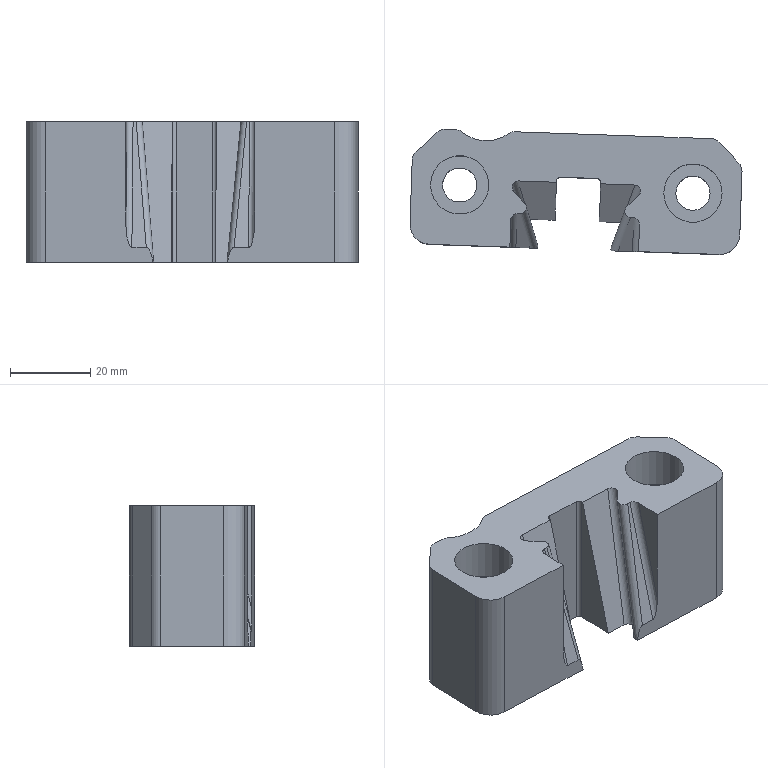Part | NX | features DIE-70 2 | 1 solid | 44 faces | box 82.504 x 31.074 x 35 mm | volume 59857 mm3 | plane 23 | cylinder 19 | spline 2 | commonest cylinder face diameters 3 x6 6 x4 2 x2 8.506 x2 10 x2 14.5 x2
STEP:
#1=CARTESIAN_POINT('',(3696.257,-880.603,858.716));
#2=VERTEX_POINT('',#1);
#3=CARTESIAN_POINT('',(3689.007,-880.603,858.716));
#4=DIRECTION('',(0.,0.,1.));
#5=DIRECTION('',(1.,0.,0.));
#6=AXIS2_PLACEMENT_3D('',#3,#4,#5);
#7=CIRCLE('',#6,7.25);
#8=EDGE_CURVE('',#2,#2,#7,.T.);
#9=ORIENTED_EDGE('',*,*,#8,.F.);
#10=EDGE_LOOP('',(#9));
#11=FACE_BOUND('',#10,.T.);
#12=CARTESIAN_POINT('',(3638.292,-878.579,858.716));
#13=VERTEX_POINT('',#12);
#14=CARTESIAN_POINT('',(3631.042,-878.579,858.716));
#15=DIRECTION('',(0.,0.,1.));
#16=DIRECTION('',(1.,0.,0.));
#17=AXIS2_PLACEMENT_3D('',#14,#15,#16);
#18=CIRCLE('',#17,7.25);
#19=EDGE_CURVE('',#13,#13,#18,.T.);
#20=ORIENTED_EDGE('',*,*,#19,.F.);
#21=EDGE_LOOP('',(#20));
#22=FACE_BOUND('',#21,.T.);
#23=CARTESIAN_POINT('',(3645.58,-877.586,858.716));
#24=VERTEX_POINT('',#23);
#25=CARTESIAN_POINT('',(3644.479,-880.196,858.716));
#26=VERTEX_POINT('',#25);
#27=CARTESIAN_POINT('',(3645.561,-879.139,858.716));
#28=DIRECTION('',(0.,0.,1.));
#29=DIRECTION('',(0.2859,-0.9583,0.));
#30=AXIS2_PLACEMENT_3D('',#27,#28,#29);
#31=ELLIPSE('',#30,1.559,1.5);
#32=EDGE_CURVE('',#24,#26,#31,.T.);
#33=ORIENTED_EDGE('',*,*,#32,.F.);
#34=CARTESIAN_POINT('',(3655.08,-877.918,858.716));
#35=VERTEX_POINT('',#34);
#36=CARTESIAN_POINT('',(3630.095,-877.045,858.716));
#37=DIRECTION('',(0.9994,-0.0349,0.));
#38=VECTOR('',#37,1000.);
#39=LINE('',#36,#38);
#40=EDGE_CURVE('',#24,#35,#39,.T.);
#41=ORIENTED_EDGE('',*,*,#40,.T.);
#42=CARTESIAN_POINT('',(3655.091,-877.612,858.716));
#43=VERTEX_POINT('',#42);
#44=CARTESIAN_POINT('',(3655.167,-875.419,858.716));
#45=DIRECTION('',(0.0349,0.9994,0.));
#46=VECTOR('',#45,1000.);
#47=LINE('',#44,#46);
#48=EDGE_CURVE('',#35,#43,#47,.T.);
#49=ORIENTED_EDGE('',*,*,#48,.T.);
#50=CARTESIAN_POINT('',(3656.125,-876.647,858.716));
#51=VERTEX_POINT('',#50);
#52=CARTESIAN_POINT('',(3656.09,-877.647,858.716));
#53=DIRECTION('',(0.,0.,1.));
#54=DIRECTION('',(1.,0.,0.));
#55=AXIS2_PLACEMENT_3D('',#52,#53,#54);
#56=CIRCLE('',#55,1.);
#57=EDGE_CURVE('',#43,#51,#56,.F.);
#58=ORIENTED_EDGE('',*,*,#57,.T.);
#59=CARTESIAN_POINT('',(3665.119,-876.962,858.716));
#60=VERTEX_POINT('',#59);
#61=CARTESIAN_POINT('',(3630.141,-875.74,858.716));
#62=DIRECTION('',(0.9994,-0.0349,0.));
#63=VECTOR('',#62,1000.);
#64=LINE('',#61,#63);
#65=EDGE_CURVE('',#51,#60,#64,.T.);
#66=ORIENTED_EDGE('',*,*,#65,.T.);
#67=CARTESIAN_POINT('',(3666.084,-877.996,858.716));
#68=VERTEX_POINT('',#67);
#69=CARTESIAN_POINT('',(3665.084,-877.961,858.716));
#70=DIRECTION('',(0.,0.,1.));
#71=DIRECTION('',(1.,0.,0.));
#72=AXIS2_PLACEMENT_3D('',#69,#70,#71);
#73=CIRCLE('',#72,1.);
#74=EDGE_CURVE('',#60,#68,#73,.F.);
#75=ORIENTED_EDGE('',*,*,#74,.T.);
#76=CARTESIAN_POINT('',(3666.073,-878.301,858.716));
#77=VERTEX_POINT('',#76);
#78=CARTESIAN_POINT('',(3666.16,-875.803,858.716));
#79=DIRECTION('',(-0.0349,-0.9994,0.));
#80=VECTOR('',#79,1000.);
#81=LINE('',#78,#80);
#82=EDGE_CURVE('',#68,#77,#81,.T.);
#83=ORIENTED_EDGE('',*,*,#82,.T.);
#84=CARTESIAN_POINT('',(3674.574,-878.598,858.716));
#85=VERTEX_POINT('',#84);
#86=CARTESIAN_POINT('',(3630.095,-877.045,858.716));
#87=DIRECTION('',(0.9994,-0.0349,0.));
#88=VECTOR('',#87,1000.);
#89=LINE('',#86,#88);
#90=EDGE_CURVE('',#77,#85,#89,.T.);
#91=ORIENTED_EDGE('',*,*,#90,.T.);
#92=CARTESIAN_POINT('',(3675.49,-881.279,858.716));
#93=VERTEX_POINT('',#92);
#94=CARTESIAN_POINT('',(3674.485,-880.149,858.716));
#95=DIRECTION('',(0.,0.,1.));
#96=DIRECTION('',(-0.352,-0.936,0.));
#97=AXIS2_PLACEMENT_3D('',#94,#95,#96);
#98=ELLIPSE('',#97,1.559,1.5);
#99=EDGE_CURVE('',#93,#85,#98,.T.);
#100=ORIENTED_EDGE('',*,*,#99,.F.);
#101=CARTESIAN_POINT('',(3672.606,-884.009,858.716));
#102=VERTEX_POINT('',#101);
#103=CARTESIAN_POINT('',(3677.106,-879.748,858.716));
#104=DIRECTION('',(0.7261,0.6876,0.));
#105=VECTOR('',#104,1000.);
#106=LINE('',#103,#105);
#107=EDGE_CURVE('',#102,#93,#106,.T.);
#108=ORIENTED_EDGE('',*,*,#107,.F.);
#109=CARTESIAN_POINT('',(3673.522,-886.69,858.716));
#110=VERTEX_POINT('',#109);
#111=CARTESIAN_POINT('',(3673.611,-885.139,858.716));
#112=DIRECTION('',(0.,0.,1.));
#113=DIRECTION('',(0.352,0.936,0.));
#114=AXIS2_PLACEMENT_3D('',#111,#112,#113);
#115=ELLIPSE('',#114,1.559,1.5);
#116=EDGE_CURVE('',#110,#102,#115,.F.);
#117=ORIENTED_EDGE('',*,*,#116,.F.);
#118=CARTESIAN_POINT('',(3674.285,-886.717,858.716));
#119=VERTEX_POINT('',#118);
#120=CARTESIAN_POINT('',(3659.756,-886.209,858.716));
#121=DIRECTION('',(-0.9994,0.0349,0.));
#122=VECTOR('',#121,1000.);
#123=LINE('',#120,#122);
#124=EDGE_CURVE('',#119,#110,#123,.T.);
#125=ORIENTED_EDGE('',*,*,#124,.F.);
#126=CARTESIAN_POINT('',(3675.729,-888.321,858.716));
#127=VERTEX_POINT('',#126);
#128=CARTESIAN_POINT('',(3674.23,-888.268,858.716));
#129=DIRECTION('',(0.,0.,1.));
#130=DIRECTION('',(-0.0349,-0.9994,0.));
#131=AXIS2_PLACEMENT_3D('',#128,#129,#130);
#132=ELLIPSE('',#131,1.553,1.5);
#133=EDGE_CURVE('',#127,#119,#132,.T.);
#134=ORIENTED_EDGE('',*,*,#133,.F.);
#135=CARTESIAN_POINT('',(3675.491,-895.14,858.716));
#136=VERTEX_POINT('',#135);
#137=CARTESIAN_POINT('',(3674.98,-909.773,858.716));
#138=DIRECTION('',(0.0349,0.9994,0.));
#139=VECTOR('',#138,1000.);
#140=LINE('',#137,#139);
#141=EDGE_CURVE('',#127,#136,#140,.F.);
#142=ORIENTED_EDGE('',*,*,#141,.T.);
#143=CARTESIAN_POINT('',(3695.479,-895.838,858.716));
#144=VERTEX_POINT('',#143);
#145=CARTESIAN_POINT('',(3629.519,-893.535,858.716));
#146=DIRECTION('',(0.9994,-0.0349,0.));
#147=VECTOR('',#146,1000.);
#148=LINE('',#145,#147);
#149=EDGE_CURVE('',#136,#144,#148,.T.);
#150=ORIENTED_EDGE('',*,*,#149,.T.);
#151=CARTESIAN_POINT('',(3700.651,-891.016,858.716));
#152=VERTEX_POINT('',#151);
#153=CARTESIAN_POINT('',(3695.654,-890.841,858.716));
#154=DIRECTION('',(0.,0.,1.));
#155=DIRECTION('',(1.,0.,0.));
#156=AXIS2_PLACEMENT_3D('',#153,#154,#155);
#157=CIRCLE('',#156,5.);
#158=EDGE_CURVE('',#144,#152,#157,.T.);
#159=ORIENTED_EDGE('',*,*,#158,.T.);
#160=CARTESIAN_POINT('',(3701.199,-875.298,858.716));
#161=VERTEX_POINT('',#160);
#162=CARTESIAN_POINT('',(3701.139,-877.024,858.716));
#163=DIRECTION('',(0.0349,0.9994,0.));
#164=VECTOR('',#163,1000.);
#165=LINE('',#162,#164);
#166=EDGE_CURVE('',#152,#161,#165,.T.);
#167=ORIENTED_EDGE('',*,*,#166,.T.);
#168=CARTESIAN_POINT('',(3700.395,-873.148,858.716));
#169=VERTEX_POINT('',#168);
#170=CARTESIAN_POINT('',(3698.201,-875.194,858.716));
#171=DIRECTION('',(0.,0.,1.));
#172=DIRECTION('',(1.,0.,0.));
#173=AXIS2_PLACEMENT_3D('',#170,#171,#172);
#174=CIRCLE('',#173,3.);
#175=EDGE_CURVE('',#161,#169,#174,.T.);
#176=ORIENTED_EDGE('',*,*,#175,.T.);
#177=CARTESIAN_POINT('',(3695.621,-868.028,858.716));
#178=VERTEX_POINT('',#177);
#179=CARTESIAN_POINT('',(3668.435,-838.875,858.716));
#180=DIRECTION('',(-0.682,0.7314,0.));
#181=VECTOR('',#180,1000.);
#182=LINE('',#179,#181);
#183=EDGE_CURVE('',#169,#178,#182,.T.);
#184=ORIENTED_EDGE('',*,*,#183,.T.);
#185=CARTESIAN_POINT('',(3693.532,-867.076,858.716));
#186=VERTEX_POINT('',#185);
#187=CARTESIAN_POINT('',(3693.427,-870.074,858.716));
#188=DIRECTION('',(0.,0.,1.));
#189=DIRECTION('',(1.,0.,0.));
#190=AXIS2_PLACEMENT_3D('',#187,#188,#189);
#191=CIRCLE('',#190,3.);
#192=EDGE_CURVE('',#178,#186,#191,.T.);
#193=ORIENTED_EDGE('',*,*,#192,.T.);
#194=CARTESIAN_POINT('',(3644.61,-865.368,858.716));
#195=VERTEX_POINT('',#194);
#196=CARTESIAN_POINT('',(3630.52,-864.876,858.716));
#197=DIRECTION('',(0.9994,-0.0349,0.));
#198=VECTOR('',#197,1000.);
#199=LINE('',#196,#198);
#200=EDGE_CURVE('',#195,#186,#199,.T.);
#201=ORIENTED_EDGE('',*,*,#200,.F.);
#202=CARTESIAN_POINT('',(3643.35,-865.759,858.716));
#203=VERTEX_POINT('',#202);
#204=CARTESIAN_POINT('',(3644.54,-867.367,858.716));
#205=DIRECTION('',(0.,0.,1.));
#206=DIRECTION('',(1.,0.,0.));
#207=AXIS2_PLACEMENT_3D('',#204,#205,#206);
#208=CIRCLE('',#207,2.);
#209=EDGE_CURVE('',#195,#203,#208,.T.);
#210=ORIENTED_EDGE('',*,*,#209,.T.);
#211=CARTESIAN_POINT('',(3631.529,-865.346,858.716));
#212=VERTEX_POINT('',#211);
#213=CARTESIAN_POINT('',(3637.699,-858.122,858.716));
#214=DIRECTION('',(0.,0.,1.));
#215=DIRECTION('',(1.,0.,0.));
#216=AXIS2_PLACEMENT_3D('',#213,#214,#215);
#217=CIRCLE('',#216,9.5);
#218=EDGE_CURVE('',#212,#203,#217,.T.);
#219=ORIENTED_EDGE('',*,*,#218,.F.);
#220=CARTESIAN_POINT('',(3630.3,-864.868,858.716));
#221=VERTEX_POINT('',#220);
#222=CARTESIAN_POINT('',(3630.23,-866.867,858.716));
#223=DIRECTION('',(0.,0.,1.));
#224=DIRECTION('',(1.,0.,0.));
#225=AXIS2_PLACEMENT_3D('',#222,#223,#224);
#226=CIRCLE('',#225,2.);
#227=EDGE_CURVE('',#212,#221,#226,.T.);
#228=ORIENTED_EDGE('',*,*,#227,.T.);
#229=CARTESIAN_POINT('',(3627.472,-864.769,858.716));
#230=VERTEX_POINT('',#229);
#231=CARTESIAN_POINT('',(3630.52,-864.876,858.716));
#232=DIRECTION('',(0.9994,-0.0349,0.));
#233=VECTOR('',#232,1000.);
#234=LINE('',#231,#233);
#235=EDGE_CURVE('',#230,#221,#234,.T.);
#236=ORIENTED_EDGE('',*,*,#235,.F.);
#237=CARTESIAN_POINT('',(3625.321,-865.574,858.716));
#238=VERTEX_POINT('',#237);
#239=CARTESIAN_POINT('',(3627.367,-867.768,858.716));
#240=DIRECTION('',(0.,0.,1.));
#241=DIRECTION('',(1.,0.,0.));
#242=AXIS2_PLACEMENT_3D('',#239,#240,#241);
#243=CIRCLE('',#242,3.);
#244=EDGE_CURVE('',#230,#238,#243,.T.);
#245=ORIENTED_EDGE('',*,*,#244,.T.);
#246=CARTESIAN_POINT('',(3620.202,-870.348,858.716));
#247=VERTEX_POINT('',#246);
#248=CARTESIAN_POINT('',(3623.446,-867.322,858.716));
#249=DIRECTION('',(-0.7314,-0.682,0.));
#250=VECTOR('',#249,1000.);
#251=LINE('',#248,#250);
#252=EDGE_CURVE('',#238,#247,#251,.T.);
#253=ORIENTED_EDGE('',*,*,#252,.T.);
#254=CARTESIAN_POINT('',(3619.249,-872.437,858.716));
#255=VERTEX_POINT('',#254);
#256=CARTESIAN_POINT('',(3622.248,-872.542,858.716));
#257=DIRECTION('',(0.,0.,1.));
#258=DIRECTION('',(1.,0.,0.));
#259=AXIS2_PLACEMENT_3D('',#256,#257,#258);
#260=CIRCLE('',#259,3.);
#261=EDGE_CURVE('',#247,#255,#260,.T.);
#262=ORIENTED_EDGE('',*,*,#261,.T.);
#263=CARTESIAN_POINT('',(3618.701,-888.154,858.716));
#264=VERTEX_POINT('',#263);
#265=CARTESIAN_POINT('',(3619.189,-874.163,858.716));
#266=DIRECTION('',(-0.0349,-0.9994,0.));
#267=VECTOR('',#266,1000.);
#268=LINE('',#265,#267);
#269=EDGE_CURVE('',#255,#264,#268,.T.);
#270=ORIENTED_EDGE('',*,*,#269,.T.);
#271=CARTESIAN_POINT('',(3623.523,-893.326,858.716));
#272=VERTEX_POINT('',#271);
#273=CARTESIAN_POINT('',(3623.697,-888.329,858.716));
#274=DIRECTION('',(0.,0.,1.));
#275=DIRECTION('',(1.,0.,0.));
#276=AXIS2_PLACEMENT_3D('',#273,#274,#275);
#277=CIRCLE('',#276,5.);
#278=EDGE_CURVE('',#264,#272,#277,.T.);
#279=ORIENTED_EDGE('',*,*,#278,.T.);
#280=CARTESIAN_POINT('',(3643.511,-894.024,858.716));
#281=VERTEX_POINT('',#280);
#282=CARTESIAN_POINT('',(3629.519,-893.535,858.716));
#283=DIRECTION('',(0.9994,-0.0349,0.));
#284=VECTOR('',#283,1000.);
#285=LINE('',#282,#284);
#286=EDGE_CURVE('',#272,#281,#285,.T.);
#287=ORIENTED_EDGE('',*,*,#286,.T.);
#288=CARTESIAN_POINT('',(3643.749,-887.204,858.716));
#289=VERTEX_POINT('',#288);
#290=CARTESIAN_POINT('',(3644.155,-875.566,858.716));
#291=DIRECTION('',(-0.0349,-0.9994,0.));
#292=VECTOR('',#291,1000.);
#293=LINE('',#290,#292);
#294=EDGE_CURVE('',#289,#281,#293,.T.);
#295=ORIENTED_EDGE('',*,*,#294,.F.);
#296=CARTESIAN_POINT('',(3645.302,-885.705,858.716));
#297=VERTEX_POINT('',#296);
#298=CARTESIAN_POINT('',(3645.248,-887.257,858.716));
#299=DIRECTION('',(0.,0.,1.));
#300=DIRECTION('',(0.0349,0.9994,0.));
#301=AXIS2_PLACEMENT_3D('',#298,#299,#300);
#302=ELLIPSE('',#301,1.553,1.5);
#303=EDGE_CURVE('',#297,#289,#302,.T.);
#304=ORIENTED_EDGE('',*,*,#303,.F.);
#305=CARTESIAN_POINT('',(3646.065,-885.731,858.716));
#306=VERTEX_POINT('',#305);
#307=CARTESIAN_POINT('',(3659.756,-886.209,858.716));
#308=DIRECTION('',(-0.9994,0.0349,0.));
#309=VECTOR('',#308,1000.);
#310=LINE('',#307,#309);
#311=EDGE_CURVE('',#306,#297,#310,.T.);
#312=ORIENTED_EDGE('',*,*,#311,.F.);
#313=CARTESIAN_POINT('',(3647.166,-883.121,858.716));
#314=VERTEX_POINT('',#313);
#315=CARTESIAN_POINT('',(3646.084,-884.178,858.716));
#316=DIRECTION('',(0.,0.,1.));
#317=DIRECTION('',(-0.2859,0.9583,0.));
#318=AXIS2_PLACEMENT_3D('',#315,#316,#317);
#319=ELLIPSE('',#318,1.559,1.5);
#320=EDGE_CURVE('',#314,#306,#319,.F.);
#321=ORIENTED_EDGE('',*,*,#320,.F.);
#322=CARTESIAN_POINT('',(3657.211,-894.061,858.716));
#323=DIRECTION('',(0.6764,-0.7365,0.));
#324=VECTOR('',#323,1000.);
#325=LINE('',#322,#324);
#326=EDGE_CURVE('',#26,#314,#325,.T.);
#327=ORIENTED_EDGE('',*,*,#326,.F.);
#328=EDGE_LOOP('',(#33,#41,#49,#58,#66,#75,#83,#91,#100,#108,#117,#125,#134,#142,#150,#159,#167,#176,#184,#193,#201,#210,#219,#228,#236,#245,#253,#262,#270,#279,#287,#295,#304,#312,#321,#327));
#329=FACE_BOUND('',#328,.T.);
#330=CARTESIAN_POINT('',(3630.182,-874.547,858.716));
#331=DIRECTION('',(0.,0.,1.));
#332=DIRECTION('',(1.,0.,0.));
#333=AXIS2_PLACEMENT_3D('',#330,#331,#332);
#334=PLANE('',#333);
#335=ADVANCED_FACE('',(#11,#22,#329),#334,.T.);
#336=CARTESIAN_POINT('',(3643.511,-894.024,833.25));
#337=VERTEX_POINT('',#336);
#338=CARTESIAN_POINT('',(3643.511,-894.024,363.715));
#339=DIRECTION('',(0.,0.,-1.));
#340=VECTOR('',#339,1000.);
#341=LINE('',#338,#340);
#342=EDGE_CURVE('',#281,#337,#341,.T.);
#343=ORIENTED_EDGE('',*,*,#342,.F.);
#344=ORIENTED_EDGE('',*,*,#286,.F.);
#345=CARTESIAN_POINT('',(3623.523,-893.326,823.716));
#346=VERTEX_POINT('',#345);
#347=CARTESIAN_POINT('',(3623.523,-893.326,363.715));
#348=DIRECTION('',(0.,0.,1.));
#349=VECTOR('',#348,1000.);
#350=LINE('',#347,#349);
#351=EDGE_CURVE('',#272,#346,#350,.F.);
#352=ORIENTED_EDGE('',*,*,#351,.T.);
#353=CARTESIAN_POINT('',(3650.313,-894.261,823.716));
#354=VERTEX_POINT('',#353);
#355=CARTESIAN_POINT('',(3615.528,-893.047,823.716));
#356=DIRECTION('',(0.9994,-0.0349,0.));
#357=VECTOR('',#356,1000.);
#358=LINE('',#355,#357);
#359=EDGE_CURVE('',#354,#346,#358,.F.);
#360=ORIENTED_EDGE('',*,*,#359,.F.);
#361=CARTESIAN_POINT('',(3648.592,-894.201,827.454));
#362=VERTEX_POINT('',#361);
#363=CARTESIAN_POINT('',(3649.079,-894.218,821.659));
#364=DIRECTION('',(-0.0349,-0.9994,0.));
#365=DIRECTION('',(-0.08981,0.003136,0.996));
#366=AXIS2_PLACEMENT_3D('',#363,#364,#365);
#367=ELLIPSE('',#366,5.818,1.5);
#368=EDGE_CURVE('',#354,#362,#367,.T.);
#369=ORIENTED_EDGE('',*,*,#368,.T.);
#370=CARTESIAN_POINT('',(3645.01,-894.076,827.454));
#371=VERTEX_POINT('',#370);
#372=CARTESIAN_POINT('',(3615.528,-893.047,827.454));
#373=DIRECTION('',(-0.9994,0.0349,0.));
#374=VECTOR('',#373,1000.);
#375=LINE('',#372,#374);
#376=EDGE_CURVE('',#362,#371,#375,.T.);
#377=ORIENTED_EDGE('',*,*,#376,.T.);
#378=CARTESIAN_POINT('',(3645.01,-894.076,833.25));
#379=DIRECTION('',(-0.0349,-0.9994,0.));
#380=DIRECTION('',(0.,0.,1.));
#381=AXIS2_PLACEMENT_3D('',#378,#379,#380);
#382=ELLIPSE('',#381,5.796,1.5);
#383=EDGE_CURVE('',#371,#337,#382,.F.);
#384=ORIENTED_EDGE('',*,*,#383,.T.);
#385=EDGE_LOOP('',(#343,#344,#352,#360,#369,#377,#384));
#386=FACE_BOUND('',#385,.T.);
#387=CARTESIAN_POINT('',(3615.528,-893.047,363.715));
#388=DIRECTION('',(-0.0349,-0.9994,0.));
#389=DIRECTION('',(0.9994,-0.0349,0.));
#390=AXIS2_PLACEMENT_3D('',#387,#388,#389);
#391=PLANE('',#390);
#392=ADVANCED_FACE('',(#386),#391,.T.);
#393=CARTESIAN_POINT('',(3684.754,-880.603,823.716));
#394=VERTEX_POINT('',#393);
#395=CARTESIAN_POINT('',(3689.007,-880.603,823.716));
#396=DIRECTION('',(0.,0.,-1.));
#397=DIRECTION('',(-1.,0.,0.));
#398=AXIS2_PLACEMENT_3D('',#395,#396,#397);
#399=CIRCLE('',#398,4.253);
#400=EDGE_CURVE('',#394,#394,#399,.T.);
#401=ORIENTED_EDGE('',*,*,#400,.F.);
#402=EDGE_LOOP('',(#401));
#403=FACE_BOUND('',#402,.T.);
#404=CARTESIAN_POINT('',(3626.789,-878.579,823.716));
#405=VERTEX_POINT('',#404);
#406=CARTESIAN_POINT('',(3631.042,-878.579,823.716));
#407=DIRECTION('',(0.,0.,-1.));
#408=DIRECTION('',(-1.,0.,0.));
#409=AXIS2_PLACEMENT_3D('',#406,#407,#408);
#410=CIRCLE('',#409,4.253);
#411=EDGE_CURVE('',#405,#405,#410,.T.);
#412=ORIENTED_EDGE('',*,*,#411,.F.);
#413=EDGE_LOOP('',(#412));
#414=FACE_BOUND('',#413,.T.);
#415=CARTESIAN_POINT('',(3649.994,-892.604,823.716));
#416=VERTEX_POINT('',#415);
#417=CARTESIAN_POINT('',(3647.308,-889.679,823.716));
#418=VERTEX_POINT('',#417);
#419=CARTESIAN_POINT('',(3685.023,-930.748,823.716));
#420=DIRECTION('',(-0.6764,0.7365,0.));
#421=VECTOR('',#420,1000.);
#422=LINE('',#419,#421);
#423=EDGE_CURVE('',#416,#418,#422,.T.);
#424=ORIENTED_EDGE('',*,*,#423,.F.);
#425=CARTESIAN_POINT('',(3648.913,-893.661,823.716));
#426=DIRECTION('',(0.,0.,-1.));
#427=DIRECTION('',(-0.2859,0.9583,0.));
#428=AXIS2_PLACEMENT_3D('',#425,#426,#427);
#429=ELLIPSE('',#428,1.559,1.5);
#430=EDGE_CURVE('',#416,#354,#429,.T.);
#431=ORIENTED_EDGE('',*,*,#430,.T.);
#432=ORIENTED_EDGE('',*,*,#359,.T.);
#433=CARTESIAN_POINT('',(3618.701,-888.154,823.716));
#434=VERTEX_POINT('',#433);
#435=CARTESIAN_POINT('',(3623.697,-888.329,823.716));
#436=DIRECTION('',(0.,0.,-1.));
#437=DIRECTION('',(-1.,0.,0.));
#438=AXIS2_PLACEMENT_3D('',#435,#436,#437);
#439=CIRCLE('',#438,5.);
#440=EDGE_CURVE('',#434,#346,#439,.F.);
#441=ORIENTED_EDGE('',*,*,#440,.F.);
#442=CARTESIAN_POINT('',(3619.249,-872.437,823.716));
#443=VERTEX_POINT('',#442);
#444=CARTESIAN_POINT('',(3619.8,-856.674,823.716));
#445=DIRECTION('',(-0.0349,-0.9994,0.));
#446=VECTOR('',#445,1000.);
#447=LINE('',#444,#446);
#448=EDGE_CURVE('',#434,#443,#447,.F.);
#449=ORIENTED_EDGE('',*,*,#448,.T.);
#450=CARTESIAN_POINT('',(3620.202,-870.348,823.716));
#451=VERTEX_POINT('',#450);
#452=CARTESIAN_POINT('',(3622.248,-872.542,823.716));
#453=DIRECTION('',(0.,0.,-1.));
#454=DIRECTION('',(-1.,0.,0.));
#455=AXIS2_PLACEMENT_3D('',#452,#453,#454);
#456=CIRCLE('',#455,3.);
#457=EDGE_CURVE('',#451,#443,#456,.F.);
#458=ORIENTED_EDGE('',*,*,#457,.F.);
#459=CARTESIAN_POINT('',(3625.321,-865.574,823.716));
#460=VERTEX_POINT('',#459);
#461=CARTESIAN_POINT('',(3636.508,-855.141,823.716));
#462=DIRECTION('',(0.7314,0.682,0.));
#463=VECTOR('',#462,1000.);
#464=LINE('',#461,#463);
#465=EDGE_CURVE('',#451,#460,#464,.T.);
#466=ORIENTED_EDGE('',*,*,#465,.T.);
#467=CARTESIAN_POINT('',(3627.472,-864.769,823.716));
#468=VERTEX_POINT('',#467);
#469=CARTESIAN_POINT('',(3627.367,-867.768,823.716));
#470=DIRECTION('',(0.,0.,-1.));
#471=DIRECTION('',(-1.,0.,0.));
#472=AXIS2_PLACEMENT_3D('',#469,#470,#471);
#473=CIRCLE('',#472,3.);
#474=EDGE_CURVE('',#468,#460,#473,.F.);
#475=ORIENTED_EDGE('',*,*,#474,.F.);
#476=CARTESIAN_POINT('',(3630.3,-864.868,823.716));
#477=VERTEX_POINT('',#476);
#478=CARTESIAN_POINT('',(3677.196,-866.506,823.716));
#479=DIRECTION('',(0.9994,-0.0349,0.));
#480=VECTOR('',#479,1000.);
#481=LINE('',#478,#480);
#482=EDGE_CURVE('',#477,#468,#481,.F.);
#483=ORIENTED_EDGE('',*,*,#482,.F.);
#484=CARTESIAN_POINT('',(3631.529,-865.346,823.716));
#485=VERTEX_POINT('',#484);
#486=CARTESIAN_POINT('',(3630.23,-866.867,823.716));
#487=DIRECTION('',(0.,0.,-1.));
#488=DIRECTION('',(-1.,0.,0.));
#489=AXIS2_PLACEMENT_3D('',#486,#487,#488);
#490=CIRCLE('',#489,2.);
#491=EDGE_CURVE('',#477,#485,#490,.T.);
#492=ORIENTED_EDGE('',*,*,#491,.T.);
#493=CARTESIAN_POINT('',(3643.351,-865.76,823.716));
#494=VERTEX_POINT('',#493);
#495=CARTESIAN_POINT('',(3643.351,-865.76,823.716));
#496=CARTESIAN_POINT('',(3641.65,-867.022,823.716));
#497=CARTESIAN_POINT('',(3637.328,-868.356,823.716));
#498=CARTESIAN_POINT('',(3633.147,-866.733,823.716));
#499=CARTESIAN_POINT('',(3631.529,-865.347,823.716));
#500=B_SPLINE_CURVE_WITH_KNOTS('',3,(#495,#496,#497,#498,#499),.UNSPECIFIED.,.F.,.F.,(4,1,4),(0.8986,1.006,1.113),.UNSPECIFIED.);
#501=EDGE_CURVE('',#485,#494,#500,.F.);
#502=ORIENTED_EDGE('',*,*,#501,.T.);
#503=CARTESIAN_POINT('',(3644.61,-865.368,823.716));
#504=VERTEX_POINT('',#503);
#505=CARTESIAN_POINT('',(3644.54,-867.367,823.716));
#506=DIRECTION('',(0.,0.,-1.));
#507=DIRECTION('',(-1.,0.,0.));
#508=AXIS2_PLACEMENT_3D('',#505,#506,#507);
#509=CIRCLE('',#508,2.);
#510=EDGE_CURVE('',#494,#504,#509,.T.);
#511=ORIENTED_EDGE('',*,*,#510,.T.);
#512=CARTESIAN_POINT('',(3693.532,-867.076,823.716));
#513=VERTEX_POINT('',#512);
#514=CARTESIAN_POINT('',(3677.196,-866.506,823.716));
#515=DIRECTION('',(0.9994,-0.0349,0.));
#516=VECTOR('',#515,1000.);
#517=LINE('',#514,#516);
#518=EDGE_CURVE('',#513,#504,#517,.F.);
#519=ORIENTED_EDGE('',*,*,#518,.F.);
#520=CARTESIAN_POINT('',(3695.621,-868.028,823.716));
#521=VERTEX_POINT('',#520);
#522=CARTESIAN_POINT('',(3693.427,-870.074,823.716));
#523=DIRECTION('',(0.,0.,-1.));
#524=DIRECTION('',(-1.,0.,0.));
#525=AXIS2_PLACEMENT_3D('',#522,#523,#524);
#526=CIRCLE('',#525,3.);
#527=EDGE_CURVE('',#513,#521,#526,.T.);
#528=ORIENTED_EDGE('',*,*,#527,.T.);
#529=CARTESIAN_POINT('',(3700.395,-873.148,823.716));
#530=VERTEX_POINT('',#529);
#531=CARTESIAN_POINT('',(3685.152,-856.802,823.716));
#532=DIRECTION('',(0.682,-0.7314,0.));
#533=VECTOR('',#532,1000.);
#534=LINE('',#531,#533);
#535=EDGE_CURVE('',#521,#530,#534,.T.);
#536=ORIENTED_EDGE('',*,*,#535,.T.);
#537=CARTESIAN_POINT('',(3701.199,-875.298,823.716));
#538=VERTEX_POINT('',#537);
#539=CARTESIAN_POINT('',(3698.201,-875.194,823.716));
#540=DIRECTION('',(0.,0.,-1.));
#541=DIRECTION('',(-1.,0.,0.));
#542=AXIS2_PLACEMENT_3D('',#539,#540,#541);
#543=CIRCLE('',#542,3.);
#544=EDGE_CURVE('',#538,#530,#543,.F.);
#545=ORIENTED_EDGE('',*,*,#544,.F.);
#546=CARTESIAN_POINT('',(3700.651,-891.016,823.716));
#547=VERTEX_POINT('',#546);
#548=CARTESIAN_POINT('',(3700.528,-894.514,823.716));
#549=DIRECTION('',(0.0349,0.9994,0.));
#550=VECTOR('',#549,1000.);
#551=LINE('',#548,#550);
#552=EDGE_CURVE('',#538,#547,#551,.F.);
#553=ORIENTED_EDGE('',*,*,#552,.T.);
#554=CARTESIAN_POINT('',(3695.479,-895.838,823.716));
#555=VERTEX_POINT('',#554);
#556=CARTESIAN_POINT('',(3695.654,-890.841,823.716));
#557=DIRECTION('',(0.,0.,-1.));
#558=DIRECTION('',(-1.,0.,0.));
#559=AXIS2_PLACEMENT_3D('',#556,#557,#558);
#560=CIRCLE('',#559,5.);
#561=EDGE_CURVE('',#547,#555,#560,.T.);
#562=ORIENTED_EDGE('',*,*,#561,.T.);
#563=CARTESIAN_POINT('',(3668.689,-894.903,823.716));
#564=VERTEX_POINT('',#563);
#565=CARTESIAN_POINT('',(3615.528,-893.047,823.716));
#566=DIRECTION('',(0.9994,-0.0349,0.));
#567=VECTOR('',#566,1000.);
#568=LINE('',#565,#567);
#569=EDGE_CURVE('',#555,#564,#568,.F.);
#570=ORIENTED_EDGE('',*,*,#569,.T.);
#571=CARTESIAN_POINT('',(3669.123,-893.272,823.716));
#572=VERTEX_POINT('',#571);
#573=CARTESIAN_POINT('',(3670.128,-894.401,823.716));
#574=DIRECTION('',(0.,0.,-1.));
#575=DIRECTION('',(0.352,0.936,0.));
#576=AXIS2_PLACEMENT_3D('',#573,#574,#575);
#577=ELLIPSE('',#576,1.559,1.5);
#578=EDGE_CURVE('',#572,#564,#577,.F.);
#579=ORIENTED_EDGE('',*,*,#578,.F.);
#580=CARTESIAN_POINT('',(3672.006,-890.541,823.716));
#581=VERTEX_POINT('',#580);
#582=CARTESIAN_POINT('',(3634.453,-926.102,823.716));
#583=DIRECTION('',(-0.7261,-0.6876,0.));
#584=VECTOR('',#583,1000.);
#585=LINE('',#582,#584);
#586=EDGE_CURVE('',#572,#581,#585,.F.);
#587=ORIENTED_EDGE('',*,*,#586,.T.);
#588=CARTESIAN_POINT('',(3671.09,-887.861,823.716));
#589=VERTEX_POINT('',#588);
#590=CARTESIAN_POINT('',(3671.001,-889.411,823.716));
#591=DIRECTION('',(0.,0.,-1.));
#592=DIRECTION('',(-0.352,-0.936,0.));
#593=AXIS2_PLACEMENT_3D('',#590,#591,#592);
#594=ELLIPSE('',#593,1.559,1.5);
#595=EDGE_CURVE('',#589,#581,#594,.T.);
#596=ORIENTED_EDGE('',*,*,#595,.F.);
#597=CARTESIAN_POINT('',(3665.746,-887.674,823.716));
#598=VERTEX_POINT('',#597);
#599=CARTESIAN_POINT('',(3659.711,-887.463,823.716));
#600=DIRECTION('',(-0.9994,0.0349,0.));
#601=VECTOR('',#600,1000.);
#602=LINE('',#599,#601);
#603=EDGE_CURVE('',#589,#598,#602,.T.);
#604=ORIENTED_EDGE('',*,*,#603,.T.);
#605=CARTESIAN_POINT('',(3666.084,-877.996,823.716));
#606=VERTEX_POINT('',#605);
#607=CARTESIAN_POINT('',(3663.364,-955.906,823.716));
#608=DIRECTION('',(-0.0349,-0.9994,0.));
#609=VECTOR('',#608,1000.);
#610=LINE('',#607,#609);
#611=EDGE_CURVE('',#606,#598,#610,.T.);
#612=ORIENTED_EDGE('',*,*,#611,.F.);
#613=CARTESIAN_POINT('',(3665.119,-876.962,823.716));
#614=VERTEX_POINT('',#613);
#615=CARTESIAN_POINT('',(3665.084,-877.961,823.716));
#616=DIRECTION('',(0.,0.,-1.));
#617=DIRECTION('',(-1.,0.,0.));
#618=AXIS2_PLACEMENT_3D('',#615,#616,#617);
#619=CIRCLE('',#618,1.);
#620=EDGE_CURVE('',#606,#614,#619,.F.);
#621=ORIENTED_EDGE('',*,*,#620,.T.);
#622=CARTESIAN_POINT('',(3656.125,-876.647,823.716));
#623=VERTEX_POINT('',#622);
#624=CARTESIAN_POINT('',(3675.113,-877.31,823.716));
#625=DIRECTION('',(0.9994,-0.0349,0.));
#626=VECTOR('',#625,1000.);
#627=LINE('',#624,#626);
#628=EDGE_CURVE('',#623,#614,#627,.T.);
#629=ORIENTED_EDGE('',*,*,#628,.F.);
#630=CARTESIAN_POINT('',(3655.091,-877.612,823.716));
#631=VERTEX_POINT('',#630);
#632=CARTESIAN_POINT('',(3656.09,-877.647,823.716));
#633=DIRECTION('',(0.,0.,-1.));
#634=DIRECTION('',(-1.,0.,0.));
#635=AXIS2_PLACEMENT_3D('',#632,#633,#634);
#636=CIRCLE('',#635,1.);
#637=EDGE_CURVE('',#623,#631,#636,.F.);
#638=ORIENTED_EDGE('',*,*,#637,.T.);
#639=CARTESIAN_POINT('',(3654.753,-887.29,823.716));
#640=VERTEX_POINT('',#639);
#641=CARTESIAN_POINT('',(3652.105,-963.113,823.716));
#642=DIRECTION('',(0.0349,0.9994,0.));
#643=VECTOR('',#642,1000.);
#644=LINE('',#641,#643);
#645=EDGE_CURVE('',#640,#631,#644,.T.);
#646=ORIENTED_EDGE('',*,*,#645,.F.);
#647=CARTESIAN_POINT('',(3648.409,-887.069,823.716));
#648=VERTEX_POINT('',#647);
#649=CARTESIAN_POINT('',(3659.711,-887.463,823.716));
#650=DIRECTION('',(-0.9994,0.0349,0.));
#651=VECTOR('',#650,1000.);
#652=LINE('',#649,#651);
#653=EDGE_CURVE('',#640,#648,#652,.T.);
#654=ORIENTED_EDGE('',*,*,#653,.T.);
#655=CARTESIAN_POINT('',(3648.39,-888.622,823.716));
#656=DIRECTION('',(0.,0.,-1.));
#657=DIRECTION('',(0.2859,-0.9583,0.));
#658=AXIS2_PLACEMENT_3D('',#655,#656,#657);
#659=ELLIPSE('',#658,1.559,1.5);
#660=EDGE_CURVE('',#418,#648,#659,.T.);
#661=ORIENTED_EDGE('',*,*,#660,.F.);
#662=EDGE_LOOP('',(#424,#431,#432,#441,#449,#458,#466,#475,#483,#492,#502,#511,#519,#528,#536,#545,#553,#562,#570,#579,#587,#596,#604,#612,#621,#629,#638,#646,#654,#661));
#663=FACE_BOUND('',#662,.T.);
#664=CARTESIAN_POINT('',(3659.962,-880.292,823.716));
#665=DIRECTION('',(0.,0.,-1.));
#666=DIRECTION('',(-1.,0.,0.));
#667=AXIS2_PLACEMENT_3D('',#664,#665,#666);
#668=PLANE('',#667);
#669=ADVANCED_FACE('',(#403,#414,#663),#668,.T.);
#670=ORIENTED_EDGE('',*,*,#235,.T.);
#671=CARTESIAN_POINT('',(3630.3,-864.868,858.716));
#672=CARTESIAN_POINT('',(3630.3,-864.868,847.05));
#673=CARTESIAN_POINT('',(3630.3,-864.868,835.383));
#674=CARTESIAN_POINT('',(3630.3,-864.868,823.716));
#675=B_SPLINE_CURVE_WITH_KNOTS('',3,(#671,#672,#673,#674),.UNSPECIFIED.,.F.,.F.,(4,4),(0.,0.035),.UNSPECIFIED.);
#676=EDGE_CURVE('',#221,#477,#675,.T.);
#677=ORIENTED_EDGE('',*,*,#676,.T.);
#678=ORIENTED_EDGE('',*,*,#482,.T.);
#679=CARTESIAN_POINT('',(3627.472,-864.769,858.716));
#680=DIRECTION('',(0.,0.,1.));
#681=VECTOR('',#680,1000.);
#682=LINE('',#679,#681);
#683=EDGE_CURVE('',#468,#230,#682,.T.);
#684=ORIENTED_EDGE('',*,*,#683,.T.);
#685=EDGE_LOOP('',(#670,#677,#678,#684));
#686=FACE_BOUND('',#685,.T.);
#687=CARTESIAN_POINT('',(3677.196,-866.506,833.716));
#688=DIRECTION('',(-0.0349,-0.9994,0.));
#689=DIRECTION('',(0.9994,-0.0349,0.));
#690=AXIS2_PLACEMENT_3D('',#687,#688,#689);
#691=PLANE('',#690);
#692=ADVANCED_FACE('',(#686),#691,.F.);
#693=CARTESIAN_POINT('',(3675.491,-895.14,833.25));
#694=VERTEX_POINT('',#693);
#695=CARTESIAN_POINT('',(3675.491,-895.14,363.715));
#696=DIRECTION('',(0.,0.,-1.));
#697=VECTOR('',#696,1000.);
#698=LINE('',#695,#697);
#699=EDGE_CURVE('',#694,#136,#698,.F.);
#700=ORIENTED_EDGE('',*,*,#699,.F.);
#701=CARTESIAN_POINT('',(3673.992,-895.088,827.454));
#702=VERTEX_POINT('',#701);
#703=CARTESIAN_POINT('',(3673.992,-895.088,833.25));
#704=DIRECTION('',(-0.0349,-0.9994,0.));
#705=DIRECTION('',(0.,0.,-1.));
#706=AXIS2_PLACEMENT_3D('',#703,#704,#705);
#707=ELLIPSE('',#706,5.796,1.5);
#708=EDGE_CURVE('',#694,#702,#707,.F.);
#709=ORIENTED_EDGE('',*,*,#708,.T.);
#710=CARTESIAN_POINT('',(3670.411,-894.963,827.454));
#711=VERTEX_POINT('',#710);
#712=CARTESIAN_POINT('',(3615.528,-893.047,827.454));
#713=DIRECTION('',(-0.9994,0.0349,0.));
#714=VECTOR('',#713,1000.);
#715=LINE('',#712,#714);
#716=EDGE_CURVE('',#702,#711,#715,.T.);
#717=ORIENTED_EDGE('',*,*,#716,.T.);
#718=CARTESIAN_POINT('',(3669.923,-894.946,821.659));
#719=DIRECTION('',(-0.0349,-0.9994,0.));
#720=DIRECTION('',(0.08981,-0.003136,0.996));
#721=AXIS2_PLACEMENT_3D('',#718,#719,#720);
#722=ELLIPSE('',#721,5.818,1.5);
#723=EDGE_CURVE('',#711,#564,#722,.T.);
#724=ORIENTED_EDGE('',*,*,#723,.T.);
#725=ORIENTED_EDGE('',*,*,#569,.F.);
#726=CARTESIAN_POINT('',(3695.479,-895.838,363.715));
#727=DIRECTION('',(0.,0.,1.));
#728=VECTOR('',#727,1000.);
#729=LINE('',#726,#728);
#730=EDGE_CURVE('',#555,#144,#729,.T.);
#731=ORIENTED_EDGE('',*,*,#730,.T.);
#732=ORIENTED_EDGE('',*,*,#149,.F.);
#733=EDGE_LOOP('',(#700,#709,#717,#724,#725,#731,#732));
#734=FACE_BOUND('',#733,.T.);
#735=CARTESIAN_POINT('',(3615.528,-893.047,363.715));
#736=DIRECTION('',(-0.0349,-0.9994,0.));
#737=DIRECTION('',(0.9994,-0.0349,0.));
#738=AXIS2_PLACEMENT_3D('',#735,#736,#737);
#739=PLANE('',#738);
#740=ADVANCED_FACE('',(#734),#739,.T.);
#741=CARTESIAN_POINT('',(3619.249,-872.437,363.715));
#742=DIRECTION('',(0.,0.,-1.));
#743=VECTOR('',#742,1000.);
#744=LINE('',#741,#743);
#745=EDGE_CURVE('',#255,#443,#744,.T.);
#746=ORIENTED_EDGE('',*,*,#745,.T.);
#747=ORIENTED_EDGE('',*,*,#448,.F.);
#748=CARTESIAN_POINT('',(3618.701,-888.154,363.715));
#749=DIRECTION('',(0.,0.,1.));
#750=VECTOR('',#749,1000.);
#751=LINE('',#748,#750);
#752=EDGE_CURVE('',#434,#264,#751,.T.);
#753=ORIENTED_EDGE('',*,*,#752,.T.);
#754=ORIENTED_EDGE('',*,*,#269,.F.);
#755=EDGE_LOOP('',(#746,#747,#753,#754));
#756=FACE_BOUND('',#755,.T.);
#757=CARTESIAN_POINT('',(3619.8,-856.674,363.715));
#758=DIRECTION('',(-0.9994,0.0349,0.));
#759=DIRECTION('',(-0.0349,-0.9994,0.));
#760=AXIS2_PLACEMENT_3D('',#757,#758,#759);
#761=PLANE('',#760);
#762=ADVANCED_FACE('',(#756),#761,.T.);
#763=CARTESIAN_POINT('',(3700.651,-891.016,363.715));
#764=DIRECTION('',(0.,0.,1.));
#765=VECTOR('',#764,1000.);
#766=LINE('',#763,#765);
#767=EDGE_CURVE('',#152,#547,#766,.F.);
#768=ORIENTED_EDGE('',*,*,#767,.T.);
#769=ORIENTED_EDGE('',*,*,#552,.F.);
#770=CARTESIAN_POINT('',(3701.199,-875.298,363.715));
#771=DIRECTION('',(0.,0.,1.));
#772=VECTOR('',#771,1000.);
#773=LINE('',#770,#772);
#774=EDGE_CURVE('',#538,#161,#773,.T.);
#775=ORIENTED_EDGE('',*,*,#774,.T.);
#776=ORIENTED_EDGE('',*,*,#166,.F.);
#777=EDGE_LOOP('',(#768,#769,#775,#776));
#778=FACE_BOUND('',#777,.T.);
#779=CARTESIAN_POINT('',(3700.528,-894.514,363.715));
#780=DIRECTION('',(0.9994,-0.0349,0.));
#781=DIRECTION('',(0.0349,0.9994,0.));
#782=AXIS2_PLACEMENT_3D('',#779,#780,#781);
#783=PLANE('',#782);
#784=ADVANCED_FACE('',(#778),#783,.T.);
#785=ORIENTED_EDGE('',*,*,#752,.F.);
#786=ORIENTED_EDGE('',*,*,#440,.T.);
#787=ORIENTED_EDGE('',*,*,#351,.F.);
#788=ORIENTED_EDGE('',*,*,#278,.F.);
#789=EDGE_LOOP('',(#785,#786,#787,#788));
#790=FACE_BOUND('',#789,.T.);
#791=CARTESIAN_POINT('',(3623.697,-888.329,363.715));
#792=DIRECTION('',(0.,0.,1.));
#793=DIRECTION('',(1.,0.,0.));
#794=AXIS2_PLACEMENT_3D('',#791,#792,#793);
#795=CYLINDRICAL_SURFACE('',#794,5.);
#796=ADVANCED_FACE('',(#790),#795,.T.);
#797=ORIENTED_EDGE('',*,*,#730,.F.);
#798=ORIENTED_EDGE('',*,*,#561,.F.);
#799=ORIENTED_EDGE('',*,*,#767,.F.);
#800=ORIENTED_EDGE('',*,*,#158,.F.);
#801=EDGE_LOOP('',(#797,#798,#799,#800));
#802=FACE_BOUND('',#801,.T.);
#803=CARTESIAN_POINT('',(3695.654,-890.841,363.715));
#804=DIRECTION('',(0.,0.,1.));
#805=DIRECTION('',(1.,0.,0.));
#806=AXIS2_PLACEMENT_3D('',#803,#804,#805);
#807=CYLINDRICAL_SURFACE('',#806,5.);
#808=ADVANCED_FACE('',(#802),#807,.T.);
#809=ORIENTED_EDGE('',*,*,#518,.T.);
#810=CARTESIAN_POINT('',(3644.61,-865.368,823.716));
#811=CARTESIAN_POINT('',(3644.61,-865.368,835.383));
#812=CARTESIAN_POINT('',(3644.61,-865.368,847.05));
#813=CARTESIAN_POINT('',(3644.61,-865.368,858.716));
#814=B_SPLINE_CURVE_WITH_KNOTS('',3,(#810,#811,#812,#813),.UNSPECIFIED.,.F.,.F.,(4,4),(0.,0.035),.UNSPECIFIED.);
#815=EDGE_CURVE('',#504,#195,#814,.T.);
#816=ORIENTED_EDGE('',*,*,#815,.T.);
#817=ORIENTED_EDGE('',*,*,#200,.T.);
#818=CARTESIAN_POINT('',(3693.532,-867.076,808.716));
#819=DIRECTION('',(0.,0.,-1.));
#820=VECTOR('',#819,1000.);
#821=LINE('',#818,#820);
#822=EDGE_CURVE('',#186,#513,#821,.T.);
#823=ORIENTED_EDGE('',*,*,#822,.T.);
#824=EDGE_LOOP('',(#809,#816,#817,#823));
#825=FACE_BOUND('',#824,.T.);
#826=CARTESIAN_POINT('',(3677.196,-866.506,833.716));
#827=DIRECTION('',(-0.0349,-0.9994,0.));
#828=DIRECTION('',(0.9994,-0.0349,0.));
#829=AXIS2_PLACEMENT_3D('',#826,#827,#828);
#830=PLANE('',#829);
#831=ADVANCED_FACE('',(#825),#830,.F.);
#832=CARTESIAN_POINT('',(3635.295,-878.579,848.716));
#833=VERTEX_POINT('',#832);
#834=CARTESIAN_POINT('',(3631.042,-878.579,848.716));
#835=DIRECTION('',(0.,0.,1.));
#836=DIRECTION('',(1.,0.,0.));
#837=AXIS2_PLACEMENT_3D('',#834,#835,#836);
#838=CIRCLE('',#837,4.253);
#839=EDGE_CURVE('',#833,#833,#838,.T.);
#840=ORIENTED_EDGE('',*,*,#839,.T.);
#841=EDGE_LOOP('',(#840));
#842=FACE_BOUND('',#841,.T.);
#843=ORIENTED_EDGE('',*,*,#411,.T.);
#844=EDGE_LOOP('',(#843));
#845=FACE_BOUND('',#844,.T.);
#846=CARTESIAN_POINT('',(3631.042,-878.579,807.716));
#847=DIRECTION('',(0.,0.,1.));
#848=DIRECTION('',(1.,0.,0.));
#849=AXIS2_PLACEMENT_3D('',#846,#847,#848);
#850=CYLINDRICAL_SURFACE('',#849,4.253);
#851=ADVANCED_FACE('',(#842,#845),#850,.F.);
#852=CARTESIAN_POINT('',(3693.26,-880.603,848.716));
#853=VERTEX_POINT('',#852);
#854=CARTESIAN_POINT('',(3689.007,-880.603,848.716));
#855=DIRECTION('',(0.,0.,1.));
#856=DIRECTION('',(1.,0.,0.));
#857=AXIS2_PLACEMENT_3D('',#854,#855,#856);
#858=CIRCLE('',#857,4.253);
#859=EDGE_CURVE('',#853,#853,#858,.T.);
#860=ORIENTED_EDGE('',*,*,#859,.T.);
#861=EDGE_LOOP('',(#860));
#862=FACE_BOUND('',#861,.T.);
#863=ORIENTED_EDGE('',*,*,#400,.T.);
#864=EDGE_LOOP('',(#863));
#865=FACE_BOUND('',#864,.T.);
#866=CARTESIAN_POINT('',(3689.007,-880.603,807.716));
#867=DIRECTION('',(0.,0.,1.));
#868=DIRECTION('',(1.,0.,0.));
#869=AXIS2_PLACEMENT_3D('',#866,#867,#868);
#870=CYLINDRICAL_SURFACE('',#869,4.253);
#871=ADVANCED_FACE('',(#862,#865),#870,.F.);
#872=CARTESIAN_POINT('',(3700.395,-873.148,363.715));
#873=DIRECTION('',(0.,0.,1.));
#874=VECTOR('',#873,1000.);
#875=LINE('',#872,#874);
#876=EDGE_CURVE('',#169,#530,#875,.F.);
#877=ORIENTED_EDGE('',*,*,#876,.T.);
#878=ORIENTED_EDGE('',*,*,#535,.F.);
#879=CARTESIAN_POINT('',(3695.621,-868.028,858.716));
#880=DIRECTION('',(0.,0.,-1.));
#881=VECTOR('',#880,1000.);
#882=LINE('',#879,#881);
#883=EDGE_CURVE('',#521,#178,#882,.F.);
#884=ORIENTED_EDGE('',*,*,#883,.T.);
#885=ORIENTED_EDGE('',*,*,#183,.F.);
#886=EDGE_LOOP('',(#877,#878,#884,#885));
#887=FACE_BOUND('',#886,.T.);
#888=CARTESIAN_POINT('',(3700.902,-873.691,363.715));
#889=DIRECTION('',(0.7314,0.682,0.));
#890=DIRECTION('',(0.,0.,-1.));
#891=AXIS2_PLACEMENT_3D('',#888,#889,#890);
#892=PLANE('',#891);
#893=ADVANCED_FACE('',(#887),#892,.T.);
#894=CARTESIAN_POINT('',(3625.321,-865.574,808.716));
#895=DIRECTION('',(0.,0.,1.));
#896=VECTOR('',#895,1000.);
#897=LINE('',#894,#896);
#898=EDGE_CURVE('',#238,#460,#897,.F.);
#899=ORIENTED_EDGE('',*,*,#898,.T.);
#900=ORIENTED_EDGE('',*,*,#465,.F.);
#901=CARTESIAN_POINT('',(3620.202,-870.348,363.715));
#902=DIRECTION('',(0.,0.,-1.));
#903=VECTOR('',#902,1000.);
#904=LINE('',#901,#903);
#905=EDGE_CURVE('',#451,#247,#904,.F.);
#906=ORIENTED_EDGE('',*,*,#905,.T.);
#907=ORIENTED_EDGE('',*,*,#252,.F.);
#908=EDGE_LOOP('',(#899,#900,#906,#907));
#909=FACE_BOUND('',#908,.T.);
#910=CARTESIAN_POINT('',(3619.658,-870.854,363.715));
#911=DIRECTION('',(-0.682,0.7314,0.));
#912=DIRECTION('',(0.,0.,1.));
#913=AXIS2_PLACEMENT_3D('',#910,#911,#912);
#914=PLANE('',#913);
#915=ADVANCED_FACE('',(#909),#914,.T.);
#916=ORIENTED_EDGE('',*,*,#883,.F.);
#917=ORIENTED_EDGE('',*,*,#527,.F.);
#918=ORIENTED_EDGE('',*,*,#822,.F.);
#919=ORIENTED_EDGE('',*,*,#192,.F.);
#920=EDGE_LOOP('',(#916,#917,#918,#919));
#921=FACE_BOUND('',#920,.T.);
#922=CARTESIAN_POINT('',(3693.427,-870.074,833.716));
#923=DIRECTION('',(0.,0.,1.));
#924=DIRECTION('',(1.,0.,0.));
#925=AXIS2_PLACEMENT_3D('',#922,#923,#924);
#926=CYLINDRICAL_SURFACE('',#925,3.);
#927=ADVANCED_FACE('',(#921),#926,.T.);
#928=ORIENTED_EDGE('',*,*,#774,.F.);
#929=ORIENTED_EDGE('',*,*,#544,.T.);
#930=ORIENTED_EDGE('',*,*,#876,.F.);
#931=ORIENTED_EDGE('',*,*,#175,.F.);
#932=EDGE_LOOP('',(#928,#929,#930,#931));
#933=FACE_BOUND('',#932,.T.);
#934=CARTESIAN_POINT('',(3698.201,-875.194,363.715));
#935=DIRECTION('',(0.,0.,1.));
#936=DIRECTION('',(1.,0.,0.));
#937=AXIS2_PLACEMENT_3D('',#934,#935,#936);
#938=CYLINDRICAL_SURFACE('',#937,3.);
#939=ADVANCED_FACE('',(#933),#938,.T.);
#940=ORIENTED_EDGE('',*,*,#683,.F.);
#941=ORIENTED_EDGE('',*,*,#474,.T.);
#942=ORIENTED_EDGE('',*,*,#898,.F.);
#943=ORIENTED_EDGE('',*,*,#244,.F.);
#944=EDGE_LOOP('',(#940,#941,#942,#943));
#945=FACE_BOUND('',#944,.T.);
#946=CARTESIAN_POINT('',(3627.367,-867.768,833.716));
#947=DIRECTION('',(0.,0.,-1.));
#948=DIRECTION('',(-1.,0.,0.));
#949=AXIS2_PLACEMENT_3D('',#946,#947,#948);
#950=CYLINDRICAL_SURFACE('',#949,3.);
#951=ADVANCED_FACE('',(#945),#950,.T.);
#952=ORIENTED_EDGE('',*,*,#905,.F.);
#953=ORIENTED_EDGE('',*,*,#457,.T.);
#954=ORIENTED_EDGE('',*,*,#745,.F.);
#955=ORIENTED_EDGE('',*,*,#261,.F.);
#956=EDGE_LOOP('',(#952,#953,#954,#955));
#957=FACE_BOUND('',#956,.T.);
#958=CARTESIAN_POINT('',(3622.248,-872.542,363.715));
#959=DIRECTION('',(0.,0.,-1.));
#960=DIRECTION('',(-1.,0.,0.));
#961=AXIS2_PLACEMENT_3D('',#958,#959,#960);
#962=CYLINDRICAL_SURFACE('',#961,3.);
#963=ADVANCED_FACE('',(#957),#962,.T.);
#964=ORIENTED_EDGE('',*,*,#19,.T.);
#965=EDGE_LOOP('',(#964));
#966=FACE_BOUND('',#965,.T.);
#967=CARTESIAN_POINT('',(3638.292,-878.579,848.716));
#968=VERTEX_POINT('',#967);
#969=CARTESIAN_POINT('',(3631.042,-878.579,848.716));
#970=DIRECTION('',(0.,0.,1.));
#971=DIRECTION('',(1.,0.,0.));
#972=AXIS2_PLACEMENT_3D('',#969,#970,#971);
#973=CIRCLE('',#972,7.25);
#974=EDGE_CURVE('',#968,#968,#973,.F.);
#975=ORIENTED_EDGE('',*,*,#974,.T.);
#976=EDGE_LOOP('',(#975));
#977=FACE_BOUND('',#976,.T.);
#978=CARTESIAN_POINT('',(3631.042,-878.579,833.716));
#979=DIRECTION('',(0.,0.,1.));
#980=DIRECTION('',(1.,0.,0.));
#981=AXIS2_PLACEMENT_3D('',#978,#979,#980);
#982=CYLINDRICAL_SURFACE('',#981,7.25);
#983=ADVANCED_FACE('',(#966,#977),#982,.F.);
#984=ORIENTED_EDGE('',*,*,#839,.F.);
#985=EDGE_LOOP('',(#984));
#986=FACE_BOUND('',#985,.T.);
#987=ORIENTED_EDGE('',*,*,#974,.F.);
#988=EDGE_LOOP('',(#987));
#989=FACE_BOUND('',#988,.T.);
#990=CARTESIAN_POINT('',(3631.042,-878.579,848.716));
#991=DIRECTION('',(0.,0.,1.));
#992=DIRECTION('',(1.,0.,0.));
#993=AXIS2_PLACEMENT_3D('',#990,#991,#992);
#994=PLANE('',#993);
#995=ADVANCED_FACE('',(#986,#989),#994,.T.);
#996=ORIENTED_EDGE('',*,*,#8,.T.);
#997=EDGE_LOOP('',(#996));
#998=FACE_BOUND('',#997,.T.);
#999=CARTESIAN_POINT('',(3696.257,-880.603,848.716));
#1000=VERTEX_POINT('',#999);
#1001=CARTESIAN_POINT('',(3689.007,-880.603,848.716));
#1002=DIRECTION('',(0.,0.,1.));
#1003=DIRECTION('',(1.,0.,0.));
#1004=AXIS2_PLACEMENT_3D('',#1001,#1002,#1003);
#1005=CIRCLE('',#1004,7.25);
#1006=EDGE_CURVE('',#1000,#1000,#1005,.F.);
#1007=ORIENTED_EDGE('',*,*,#1006,.T.);
#1008=EDGE_LOOP('',(#1007));
#1009=FACE_BOUND('',#1008,.T.);
#1010=CARTESIAN_POINT('',(3689.007,-880.603,833.716));
#1011=DIRECTION('',(0.,0.,1.));
#1012=DIRECTION('',(1.,0.,0.));
#1013=AXIS2_PLACEMENT_3D('',#1010,#1011,#1012);
#1014=CYLINDRICAL_SURFACE('',#1013,7.25);
#1015=ADVANCED_FACE('',(#998,#1009),#1014,.F.);
#1016=ORIENTED_EDGE('',*,*,#859,.F.);
#1017=EDGE_LOOP('',(#1016));
#1018=FACE_BOUND('',#1017,.T.);
#1019=ORIENTED_EDGE('',*,*,#1006,.F.);
#1020=EDGE_LOOP('',(#1019));
#1021=FACE_BOUND('',#1020,.T.);
#1022=CARTESIAN_POINT('',(3689.007,-880.603,848.716));
#1023=DIRECTION('',(0.,0.,1.));
#1024=DIRECTION('',(1.,0.,0.));
#1025=AXIS2_PLACEMENT_3D('',#1022,#1023,#1024);
#1026=PLANE('',#1025);
#1027=ADVANCED_FACE('',(#1018,#1021),#1026,.T.);
#1028=ORIENTED_EDGE('',*,*,#218,.T.);
#1029=CARTESIAN_POINT('',(3643.35,-865.759,858.716));
#1030=CARTESIAN_POINT('',(3643.35,-865.759,847.05));
#1031=CARTESIAN_POINT('',(3643.35,-865.759,835.383));
#1032=CARTESIAN_POINT('',(3643.35,-865.759,823.716));
#1033=B_SPLINE_CURVE_WITH_KNOTS('',3,(#1029,#1030,#1031,#1032),.UNSPECIFIED.,.F.,.F.,(4,4),(0.,0.035),.UNSPECIFIED.);
#1034=EDGE_CURVE('',#203,#494,#1033,.T.);
#1035=ORIENTED_EDGE('',*,*,#1034,.T.);
#1036=ORIENTED_EDGE('',*,*,#501,.F.);
#1037=CARTESIAN_POINT('',(3631.529,-865.346,823.716));
#1038=CARTESIAN_POINT('',(3631.529,-865.346,835.383));
#1039=CARTESIAN_POINT('',(3631.529,-865.346,847.05));
#1040=CARTESIAN_POINT('',(3631.529,-865.346,858.716));
#1041=B_SPLINE_CURVE_WITH_KNOTS('',3,(#1037,#1038,#1039,#1040),.UNSPECIFIED.,.F.,.F.,(4,4),(0.,0.035),.UNSPECIFIED.);
#1042=EDGE_CURVE('',#485,#212,#1041,.T.);
#1043=ORIENTED_EDGE('',*,*,#1042,.T.);
#1044=EDGE_LOOP('',(#1028,#1035,#1036,#1043));
#1045=FACE_BOUND('',#1044,.T.);
#1046=CARTESIAN_POINT('',(3637.699,-858.122,802.716));
#1047=DIRECTION('',(0.,0.000000057,1.));
#1048=DIRECTION('',(1.,0.,0.));
#1049=AXIS2_PLACEMENT_3D('',#1046,#1047,#1048);
#1050=CYLINDRICAL_SURFACE('',#1049,9.5);
#1051=ADVANCED_FACE('',(#1045),#1050,.F.);
#1052=ORIENTED_EDGE('',*,*,#510,.F.);
#1053=ORIENTED_EDGE('',*,*,#1034,.F.);
#1054=ORIENTED_EDGE('',*,*,#209,.F.);
#1055=ORIENTED_EDGE('',*,*,#815,.F.);
#1056=EDGE_LOOP('',(#1052,#1053,#1054,#1055));
#1057=FACE_BOUND('',#1056,.T.);
#1058=CARTESIAN_POINT('',(3644.61,-865.368,858.716));
#1059=CARTESIAN_POINT('',(3643.912,-865.344,858.716));
#1060=CARTESIAN_POINT('',(3643.35,-865.759,858.716));
#1061=CARTESIAN_POINT('',(3644.61,-865.368,847.05));
#1062=CARTESIAN_POINT('',(3643.911,-865.343,847.05));
#1063=CARTESIAN_POINT('',(3643.35,-865.759,847.05));
#1064=CARTESIAN_POINT('',(3644.61,-865.368,835.383));
#1065=CARTESIAN_POINT('',(3643.912,-865.344,835.383));
#1066=CARTESIAN_POINT('',(3643.35,-865.759,835.383));
#1067=CARTESIAN_POINT('',(3644.61,-865.368,823.716));
#1068=CARTESIAN_POINT('',(3643.912,-865.344,823.716));
#1069=CARTESIAN_POINT('',(3643.35,-865.759,823.716));
#1070=(BOUNDED_SURFACE()B_SPLINE_SURFACE(3,2,((#1058,#1059,#1060),(#1061,#1062,#1063),(#1064,#1065,#1066),(#1067,#1068,#1069)),.UNSPECIFIED.,.F.,.F.,.F.)B_SPLINE_SURFACE_WITH_KNOTS((4,4),(3,3),(0.007001,0.042),(0.,1.),.PIECEWISE_BEZIER_KNOTS.)GEOMETRIC_REPRESENTATION_ITEM()RATIONAL_B_SPLINE_SURFACE(((1.,0.9441,1.),(1.,0.9441,1.),(1.,0.9441,1.),(1.,0.9441,1.)))REPRESENTATION_ITEM('')SURFACE());
#1071=ADVANCED_FACE('',(#1057),#1070,.T.);
#1072=ORIENTED_EDGE('',*,*,#227,.F.);
#1073=ORIENTED_EDGE('',*,*,#1042,.F.);
#1074=ORIENTED_EDGE('',*,*,#491,.F.);
#1075=ORIENTED_EDGE('',*,*,#676,.F.);
#1076=EDGE_LOOP('',(#1072,#1073,#1074,#1075));
#1077=FACE_BOUND('',#1076,.T.);
#1078=CARTESIAN_POINT('',(3631.529,-865.346,858.716));
#1079=CARTESIAN_POINT('',(3630.998,-864.893,858.716));
#1080=CARTESIAN_POINT('',(3630.3,-864.868,858.716));
#1081=CARTESIAN_POINT('',(3631.529,-865.346,847.05));
#1082=CARTESIAN_POINT('',(3630.998,-864.893,847.05));
#1083=CARTESIAN_POINT('',(3630.3,-864.868,847.05));
#1084=CARTESIAN_POINT('',(3631.529,-865.346,835.383));
#1085=CARTESIAN_POINT('',(3630.998,-864.893,835.383));
#1086=CARTESIAN_POINT('',(3630.3,-864.868,835.383));
#1087=CARTESIAN_POINT('',(3631.529,-865.346,823.716));
#1088=CARTESIAN_POINT('',(3630.998,-864.893,823.716));
#1089=CARTESIAN_POINT('',(3630.3,-864.868,823.716));
#1090=(BOUNDED_SURFACE()B_SPLINE_SURFACE(3,2,((#1078,#1079,#1080),(#1081,#1082,#1083),(#1084,#1085,#1086),(#1087,#1088,#1089)),.UNSPECIFIED.,.F.,.F.,.F.)B_SPLINE_SURFACE_WITH_KNOTS((4,4),(3,3),(0.004,0.039),(0.,1.),.PIECEWISE_BEZIER_KNOTS.)GEOMETRIC_REPRESENTATION_ITEM()RATIONAL_B_SPLINE_SURFACE(((1.,0.9441,1.),(1.,0.9441,1.),(1.,0.9441,1.),(1.,0.9441,1.)))REPRESENTATION_ITEM('')SURFACE());
#1091=ADVANCED_FACE('',(#1077),#1090,.T.);
#1092=ORIENTED_EDGE('',*,*,#40,.F.);
#1093=CARTESIAN_POINT('',(3645.678,-877.913,857.507));
#1094=DIRECTION('',(0.07778,-0.2607,-0.9623));
#1095=VECTOR('',#1094,1000.);
#1096=LINE('',#1093,#1095);
#1097=EDGE_CURVE('',#24,#648,#1096,.T.);
#1098=ORIENTED_EDGE('',*,*,#1097,.T.);
#1099=ORIENTED_EDGE('',*,*,#653,.F.);
#1100=CARTESIAN_POINT('',(3650.663,-1004.416,386.329));
#1101=DIRECTION('',(-0.009032,-0.2587,-0.9659));
#1102=VECTOR('',#1101,1000.);
#1103=LINE('',#1100,#1102);
#1104=EDGE_CURVE('',#35,#640,#1103,.T.);
#1105=ORIENTED_EDGE('',*,*,#1104,.F.);
#1106=EDGE_LOOP('',(#1092,#1098,#1099,#1105));
#1107=FACE_BOUND('',#1106,.T.);
#1108=CARTESIAN_POINT('',(3660.039,-878.091,858.716));
#1109=DIRECTION('',(-0.03371,-0.9653,0.2588));
#1110=DIRECTION('',(0.,-0.259,-0.9659));
#1111=AXIS2_PLACEMENT_3D('',#1108,#1109,#1110);
#1112=PLANE('',#1111);
#1113=ADVANCED_FACE('',(#1107),#1112,.T.);
#1114=CARTESIAN_POINT('',(3674.453,-878.92,857.501));
#1115=DIRECTION('',(0.09577,0.2547,0.9623));
#1116=VECTOR('',#1115,1000.);
#1117=LINE('',#1114,#1116);
#1118=EDGE_CURVE('',#85,#589,#1117,.F.);
#1119=ORIENTED_EDGE('',*,*,#1118,.F.);
#1120=ORIENTED_EDGE('',*,*,#90,.F.);
#1121=CARTESIAN_POINT('',(3666.073,-878.301,858.716));
#1122=DIRECTION('',(-0.009032,-0.2587,-0.9659));
#1123=VECTOR('',#1122,1000.);
#1124=LINE('',#1121,#1123);
#1125=EDGE_CURVE('',#77,#598,#1124,.T.);
#1126=ORIENTED_EDGE('',*,*,#1125,.T.);
#1127=ORIENTED_EDGE('',*,*,#603,.F.);
#1128=EDGE_LOOP('',(#1119,#1120,#1126,#1127));
#1129=FACE_BOUND('',#1128,.T.);
#1130=CARTESIAN_POINT('',(3660.039,-878.091,858.716));
#1131=DIRECTION('',(-0.03371,-0.9653,0.2588));
#1132=DIRECTION('',(0.,-0.259,-0.9659));
#1133=AXIS2_PLACEMENT_3D('',#1130,#1131,#1132);
#1134=PLANE('',#1133);
#1135=ADVANCED_FACE('',(#1129),#1134,.T.);
#1136=ORIENTED_EDGE('',*,*,#660,.T.);
#1137=ORIENTED_EDGE('',*,*,#1097,.F.);
#1138=ORIENTED_EDGE('',*,*,#32,.T.);
#1139=CARTESIAN_POINT('',(3682.375,-1007.226,389.856));
#1140=DIRECTION('',(0.07778,-0.2607,-0.9623));
#1141=VECTOR('',#1140,1000.);
#1142=LINE('',#1139,#1141);
#1143=EDGE_CURVE('',#418,#26,#1142,.F.);
#1144=ORIENTED_EDGE('',*,*,#1143,.F.);
#1145=EDGE_LOOP('',(#1136,#1137,#1138,#1144));
#1146=FACE_BOUND('',#1145,.T.);
#1147=CARTESIAN_POINT('',(3683.471,-1006.219,389.672));
#1148=DIRECTION('',(0.07778,-0.2607,-0.9623));
#1149=DIRECTION('',(0.,0.9652,-0.2615));
#1150=AXIS2_PLACEMENT_3D('',#1147,#1148,#1149);
#1151=CYLINDRICAL_SURFACE('',#1150,1.5);
#1152=ADVANCED_FACE('',(#1146),#1151,.F.);
#1153=ORIENTED_EDGE('',*,*,#595,.T.);
#1154=CARTESIAN_POINT('',(3675.426,-881.449,858.074));
#1155=DIRECTION('',(0.09577,0.2547,0.9623));
#1156=VECTOR('',#1155,1000.);
#1157=LINE('',#1154,#1156);
#1158=EDGE_CURVE('',#581,#93,#1157,.T.);
#1159=ORIENTED_EDGE('',*,*,#1158,.T.);
#1160=ORIENTED_EDGE('',*,*,#99,.T.);
#1161=ORIENTED_EDGE('',*,*,#1118,.T.);
#1162=EDGE_LOOP('',(#1153,#1159,#1160,#1161));
#1163=FACE_BOUND('',#1162,.T.);
#1164=CARTESIAN_POINT('',(3674.402,-880.368,857.889));
#1165=DIRECTION('',(-0.09577,-0.2547,-0.9623));
#1166=DIRECTION('',(0.,0.9667,-0.2558));
#1167=AXIS2_PLACEMENT_3D('',#1164,#1165,#1166);
#1168=CYLINDRICAL_SURFACE('',#1167,1.5);
#1169=ADVANCED_FACE('',(#1163),#1168,.F.);
#1170=ORIENTED_EDGE('',*,*,#699,.T.);
#1171=ORIENTED_EDGE('',*,*,#141,.F.);
#1172=CARTESIAN_POINT('',(3675.733,-888.217,859.105));
#1173=DIRECTION('',(-0.009032,-0.2587,-0.9659));
#1174=VECTOR('',#1173,1000.);
#1175=LINE('',#1172,#1174);
#1176=EDGE_CURVE('',#127,#694,#1175,.T.);
#1177=ORIENTED_EDGE('',*,*,#1176,.T.);
#1178=EDGE_LOOP('',(#1170,#1171,#1177));
#1179=FACE_BOUND('',#1178,.T.);
#1180=CARTESIAN_POINT('',(3674.98,-909.773,891.507));
#1181=DIRECTION('',(-0.9994,0.0349,0.));
#1182=DIRECTION('',(-0.0349,-0.9994,0.));
#1183=AXIS2_PLACEMENT_3D('',#1180,#1181,#1182);
#1184=PLANE('',#1183);
#1185=ADVANCED_FACE('',(#1179),#1184,.T.);
#1186=ORIENTED_EDGE('',*,*,#342,.T.);
#1187=CARTESIAN_POINT('',(3644.492,-865.919,938.203));
#1188=DIRECTION('',(0.009032,0.2587,0.9659));
#1189=VECTOR('',#1188,1000.);
#1190=LINE('',#1187,#1189);
#1191=EDGE_CURVE('',#289,#337,#1190,.F.);
#1192=ORIENTED_EDGE('',*,*,#1191,.F.);
#1193=ORIENTED_EDGE('',*,*,#294,.T.);
#1194=EDGE_LOOP('',(#1186,#1192,#1193));
#1195=FACE_BOUND('',#1194,.T.);
#1196=CARTESIAN_POINT('',(3643.206,-902.74,948.075));
#1197=DIRECTION('',(-0.9994,0.0349,0.));
#1198=DIRECTION('',(-0.0349,-0.9994,0.));
#1199=AXIS2_PLACEMENT_3D('',#1196,#1197,#1198);
#1200=PLANE('',#1199);
#1201=ADVANCED_FACE('',(#1195),#1200,.F.);
#1202=ORIENTED_EDGE('',*,*,#65,.F.);
#1203=CARTESIAN_POINT('',(3656.125,-876.647,823.716));
#1204=DIRECTION('',(0.,0.,-1.));
#1205=VECTOR('',#1204,1000.);
#1206=LINE('',#1203,#1205);
#1207=EDGE_CURVE('',#51,#623,#1206,.T.);
#1208=ORIENTED_EDGE('',*,*,#1207,.T.);
#1209=ORIENTED_EDGE('',*,*,#628,.T.);
#1210=CARTESIAN_POINT('',(3665.119,-876.962,858.716));
#1211=DIRECTION('',(0.,0.,1.));
#1212=VECTOR('',#1211,1000.);
#1213=LINE('',#1210,#1212);
#1214=EDGE_CURVE('',#614,#60,#1213,.T.);
#1215=ORIENTED_EDGE('',*,*,#1214,.T.);
#1216=EDGE_LOOP('',(#1202,#1208,#1209,#1215));
#1217=FACE_BOUND('',#1216,.T.);
#1218=CARTESIAN_POINT('',(3675.113,-877.31,820.307));
#1219=DIRECTION('',(-0.0349,-0.9994,0.));
#1220=DIRECTION('',(0.9994,-0.0349,0.));
#1221=AXIS2_PLACEMENT_3D('',#1218,#1219,#1220);
#1222=PLANE('',#1221);
#1223=ADVANCED_FACE('',(#1217),#1222,.T.);
#1224=ORIENTED_EDGE('',*,*,#1191,.T.);
#1225=ORIENTED_EDGE('',*,*,#383,.F.);
#1226=CARTESIAN_POINT('',(3645.302,-885.705,858.716));
#1227=DIRECTION('',(0.009032,0.2587,0.9659));
#1228=VECTOR('',#1227,1000.);
#1229=LINE('',#1226,#1228);
#1230=EDGE_CURVE('',#371,#297,#1229,.T.);
#1231=ORIENTED_EDGE('',*,*,#1230,.T.);
#1232=ORIENTED_EDGE('',*,*,#303,.T.);
#1233=EDGE_LOOP('',(#1224,#1225,#1231,#1232));
#1234=FACE_BOUND('',#1233,.T.);
#1235=CARTESIAN_POINT('',(3645.991,-865.971,938.203));
#1236=DIRECTION('',(0.009032,0.2587,0.9659));
#1237=DIRECTION('',(0.,-0.966,0.2587));
#1238=AXIS2_PLACEMENT_3D('',#1235,#1236,#1237);
#1239=CYLINDRICAL_SURFACE('',#1238,1.5);
#1240=ADVANCED_FACE('',(#1234),#1239,.F.);
#1241=ORIENTED_EDGE('',*,*,#423,.T.);
#1242=ORIENTED_EDGE('',*,*,#1143,.T.);
#1243=ORIENTED_EDGE('',*,*,#326,.T.);
#1244=CARTESIAN_POINT('',(3684.986,-1009.898,390.791));
#1245=DIRECTION('',(-0.07778,0.2607,0.9623));
#1246=VECTOR('',#1245,1000.);
#1247=LINE('',#1244,#1246);
#1248=EDGE_CURVE('',#416,#314,#1247,.T.);
#1249=ORIENTED_EDGE('',*,*,#1248,.F.);
#1250=EDGE_LOOP('',(#1241,#1242,#1243,#1249));
#1251=FACE_BOUND('',#1250,.T.);
#1252=CARTESIAN_POINT('',(3644.241,-968.198,376.2));
#1253=DIRECTION('',(0.731,0.6713,-0.1228));
#1254=DIRECTION('',(-0.6764,0.7365,0.));
#1255=AXIS2_PLACEMENT_3D('',#1252,#1253,#1254);
#1256=PLANE('',#1255);
#1257=ADVANCED_FACE('',(#1251),#1256,.T.);
#1258=ORIENTED_EDGE('',*,*,#430,.F.);
#1259=ORIENTED_EDGE('',*,*,#1248,.T.);
#1260=ORIENTED_EDGE('',*,*,#320,.T.);
#1261=CARTESIAN_POINT('',(3646.157,-886.041,857.572));
#1262=DIRECTION('',(0.07778,-0.2607,-0.9623));
#1263=VECTOR('',#1262,1000.);
#1264=LINE('',#1261,#1263);
#1265=EDGE_CURVE('',#362,#306,#1264,.F.);
#1266=ORIENTED_EDGE('',*,*,#1265,.F.);
#1267=ORIENTED_EDGE('',*,*,#368,.F.);
#1268=EDGE_LOOP('',(#1258,#1259,#1260,#1266,#1267));
#1269=FACE_BOUND('',#1268,.T.);
#1270=CARTESIAN_POINT('',(3646.208,-884.593,857.183));
#1271=DIRECTION('',(-0.07778,0.2607,0.9623));
#1272=DIRECTION('',(0.,-0.9652,0.2615));
#1273=AXIS2_PLACEMENT_3D('',#1270,#1271,#1272);
#1274=CYLINDRICAL_SURFACE('',#1273,1.5);
#1275=ADVANCED_FACE('',(#1269),#1274,.T.);
#1276=ORIENTED_EDGE('',*,*,#1265,.T.);
#1277=ORIENTED_EDGE('',*,*,#311,.T.);
#1278=ORIENTED_EDGE('',*,*,#1230,.F.);
#1279=ORIENTED_EDGE('',*,*,#376,.F.);
#1280=EDGE_LOOP('',(#1276,#1277,#1278,#1279));
#1281=FACE_BOUND('',#1280,.T.);
#1282=CARTESIAN_POINT('',(3659.756,-886.209,858.716));
#1283=DIRECTION('',(-0.03371,-0.9653,0.2588));
#1284=DIRECTION('',(0.,-0.259,-0.9659));
#1285=AXIS2_PLACEMENT_3D('',#1282,#1283,#1284);
#1286=PLANE('',#1285);
#1287=ADVANCED_FACE('',(#1281),#1286,.T.);
#1288=ORIENTED_EDGE('',*,*,#645,.T.);
#1289=CARTESIAN_POINT('',(3655.091,-877.612,858.716));
#1290=DIRECTION('',(0.,0.,-1.));
#1291=VECTOR('',#1290,1000.);
#1292=LINE('',#1289,#1291);
#1293=EDGE_CURVE('',#631,#43,#1292,.F.);
#1294=ORIENTED_EDGE('',*,*,#1293,.T.);
#1295=ORIENTED_EDGE('',*,*,#48,.F.);
#1296=ORIENTED_EDGE('',*,*,#1104,.T.);
#1297=EDGE_LOOP('',(#1288,#1294,#1295,#1296));
#1298=FACE_BOUND('',#1297,.T.);
#1299=CARTESIAN_POINT('',(3652.105,-963.113,375.255));
#1300=DIRECTION('',(0.9994,-0.0349,0.));
#1301=DIRECTION('',(0.0349,0.9994,0.));
#1302=AXIS2_PLACEMENT_3D('',#1299,#1300,#1301);
#1303=PLANE('',#1302);
#1304=ADVANCED_FACE('',(#1298),#1303,.T.);
#1305=ORIENTED_EDGE('',*,*,#82,.F.);
#1306=CARTESIAN_POINT('',(3666.084,-877.996,823.716));
#1307=DIRECTION('',(0.,0.,1.));
#1308=VECTOR('',#1307,1000.);
#1309=LINE('',#1306,#1308);
#1310=EDGE_CURVE('',#68,#606,#1309,.F.);
#1311=ORIENTED_EDGE('',*,*,#1310,.T.);
#1312=ORIENTED_EDGE('',*,*,#611,.T.);
#1313=ORIENTED_EDGE('',*,*,#1125,.F.);
#1314=EDGE_LOOP('',(#1305,#1311,#1312,#1313));
#1315=FACE_BOUND('',#1314,.T.);
#1316=CARTESIAN_POINT('',(3663.364,-955.906,373.916));
#1317=DIRECTION('',(-0.9994,0.0349,0.));
#1318=DIRECTION('',(-0.0349,-0.9994,0.));
#1319=AXIS2_PLACEMENT_3D('',#1316,#1317,#1318);
#1320=PLANE('',#1319);
#1321=ADVANCED_FACE('',(#1315),#1320,.T.);
#1322=ORIENTED_EDGE('',*,*,#586,.F.);
#1323=CARTESIAN_POINT('',(3626.083,-1007.713,391.272));
#1324=DIRECTION('',(-0.09577,-0.2547,-0.9623));
#1325=VECTOR('',#1324,1000.);
#1326=LINE('',#1323,#1325);
#1327=EDGE_CURVE('',#572,#102,#1326,.F.);
#1328=ORIENTED_EDGE('',*,*,#1327,.T.);
#1329=ORIENTED_EDGE('',*,*,#107,.T.);
#1330=ORIENTED_EDGE('',*,*,#1158,.F.);
#1331=EDGE_LOOP('',(#1322,#1328,#1329,#1330));
#1332=FACE_BOUND('',#1331,.T.);
#1333=CARTESIAN_POINT('',(3672.565,-966.351,375.7));
#1334=DIRECTION('',(-0.6824,0.7206,-0.1228));
#1335=DIRECTION('',(-0.7261,-0.6876,0.));
#1336=AXIS2_PLACEMENT_3D('',#1333,#1334,#1335);
#1337=PLANE('',#1336);
#1338=ADVANCED_FACE('',(#1332),#1337,.T.);
#1339=CARTESIAN_POINT('',(3673.407,-886.994,857.565));
#1340=DIRECTION('',(0.09577,0.2547,0.9623));
#1341=VECTOR('',#1340,1000.);
#1342=LINE('',#1339,#1341);
#1343=EDGE_CURVE('',#711,#110,#1342,.T.);
#1344=ORIENTED_EDGE('',*,*,#1343,.T.);
#1345=ORIENTED_EDGE('',*,*,#116,.T.);
#1346=ORIENTED_EDGE('',*,*,#1327,.F.);
#1347=ORIENTED_EDGE('',*,*,#578,.T.);
#1348=ORIENTED_EDGE('',*,*,#723,.F.);
#1349=EDGE_LOOP('',(#1344,#1345,#1346,#1347,#1348));
#1350=FACE_BOUND('',#1349,.T.);
#1351=CARTESIAN_POINT('',(3627.107,-1008.794,391.456));
#1352=DIRECTION('',(0.09577,0.2547,0.9623));
#1353=DIRECTION('',(0.,-0.9667,0.2558));
#1354=AXIS2_PLACEMENT_3D('',#1351,#1352,#1353);
#1355=CYLINDRICAL_SURFACE('',#1354,1.5);
#1356=ADVANCED_FACE('',(#1350),#1355,.T.);
#1357=ORIENTED_EDGE('',*,*,#124,.T.);
#1358=ORIENTED_EDGE('',*,*,#1343,.F.);
#1359=ORIENTED_EDGE('',*,*,#716,.F.);
#1360=CARTESIAN_POINT('',(3674.285,-886.717,858.716));
#1361=DIRECTION('',(0.009032,0.2587,0.9659));
#1362=VECTOR('',#1361,1000.);
#1363=LINE('',#1360,#1362);
#1364=EDGE_CURVE('',#702,#119,#1363,.T.);
#1365=ORIENTED_EDGE('',*,*,#1364,.T.);
#1366=EDGE_LOOP('',(#1357,#1358,#1359,#1365));
#1367=FACE_BOUND('',#1366,.T.);
#1368=CARTESIAN_POINT('',(3659.756,-886.209,858.716));
#1369=DIRECTION('',(-0.03371,-0.9653,0.2588));
#1370=DIRECTION('',(0.,-0.259,-0.9659));
#1371=AXIS2_PLACEMENT_3D('',#1368,#1369,#1370);
#1372=PLANE('',#1371);
#1373=ADVANCED_FACE('',(#1367),#1372,.T.);
#1374=ORIENTED_EDGE('',*,*,#708,.F.);
#1375=ORIENTED_EDGE('',*,*,#1176,.F.);
#1376=ORIENTED_EDGE('',*,*,#133,.T.);
#1377=ORIENTED_EDGE('',*,*,#1364,.F.);
#1378=EDGE_LOOP('',(#1374,#1375,#1376,#1377));
#1379=FACE_BOUND('',#1378,.T.);
#1380=CARTESIAN_POINT('',(3674.234,-888.165,859.105));
#1381=DIRECTION('',(-0.009032,-0.2587,-0.9659));
#1382=DIRECTION('',(0.,0.966,-0.2587));
#1383=AXIS2_PLACEMENT_3D('',#1380,#1381,#1382);
#1384=CYLINDRICAL_SURFACE('',#1383,1.5);
#1385=ADVANCED_FACE('',(#1379),#1384,.F.);
#1386=ORIENTED_EDGE('',*,*,#57,.F.);
#1387=ORIENTED_EDGE('',*,*,#1293,.F.);
#1388=ORIENTED_EDGE('',*,*,#637,.F.);
#1389=ORIENTED_EDGE('',*,*,#1207,.F.);
#1390=EDGE_LOOP('',(#1386,#1387,#1388,#1389));
#1391=FACE_BOUND('',#1390,.T.);
#1392=CARTESIAN_POINT('',(3656.09,-877.647,820.307));
#1393=DIRECTION('',(0.,0.,1.));
#1394=DIRECTION('',(1.,0.,0.));
#1395=AXIS2_PLACEMENT_3D('',#1392,#1393,#1394);
#1396=CYLINDRICAL_SURFACE('',#1395,1.);
#1397=ADVANCED_FACE('',(#1391),#1396,.F.);
#1398=ORIENTED_EDGE('',*,*,#620,.F.);
#1399=ORIENTED_EDGE('',*,*,#1310,.F.);
#1400=ORIENTED_EDGE('',*,*,#74,.F.);
#1401=ORIENTED_EDGE('',*,*,#1214,.F.);
#1402=EDGE_LOOP('',(#1398,#1399,#1400,#1401));
#1403=FACE_BOUND('',#1402,.T.);
#1404=CARTESIAN_POINT('',(3665.084,-877.961,820.307));
#1405=DIRECTION('',(0.,0.,-1.));
#1406=DIRECTION('',(-1.,0.,0.));
#1407=AXIS2_PLACEMENT_3D('',#1404,#1405,#1406);
#1408=CYLINDRICAL_SURFACE('',#1407,1.);
#1409=ADVANCED_FACE('',(#1403),#1408,.F.);
#1410=CLOSED_SHELL('',(#335,#392,#669,#692,#740,#762,#784,#796,#808,#831,#851,#871,#893,#915,#927,#939,#951,#963,#983,#995,#1015,#1027,#1051,#1071,#1091,#1113,#1135,#1152,#1169,#1185,#1201,#1223,#1240,#1257,#1275,#1287,#1304,#1321,#1338,#1356,#1373,#1385,#1397,#1409));
#1411=MANIFOLD_SOLID_BREP('',#1410);
#1412=(LENGTH_UNIT()NAMED_UNIT(*)SI_UNIT(.MILLI.,.METRE.));
#1413=UNCERTAINTY_MEASURE_WITH_UNIT(LENGTH_MEASURE(0.0508),#1412,'','');
#1414=(NAMED_UNIT(*)PLANE_ANGLE_UNIT()SI_UNIT($,.RADIAN.));
#1415=(NAMED_UNIT(*)SI_UNIT($,.STERADIAN.)SOLID_ANGLE_UNIT());
#1416=(GEOMETRIC_REPRESENTATION_CONTEXT(3)GLOBAL_UNCERTAINTY_ASSIGNED_CONTEXT((#1413))GLOBAL_UNIT_ASSIGNED_CONTEXT((#1412,#1414,#1415))REPRESENTATION_CONTEXT('',''));
#1417=ADVANCED_BREP_SHAPE_REPRESENTATION('',(#1411),#1416);